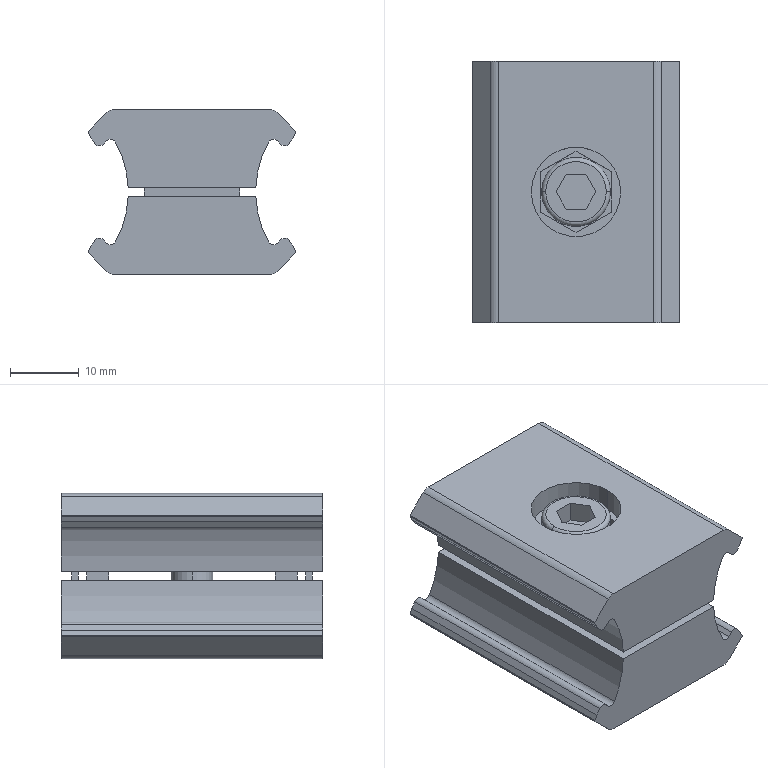Part | STEP file | 1 solid | 124 faces | box 30.2 x 38 x 24 mm | volume 19567 mm3 | plane 76 | cylinder 32 | cone 14 | torus 2 | commonest cylinder face diameters 1.6 x8 11.05 x6 3 x4 6 x4 13 x4 30 x4